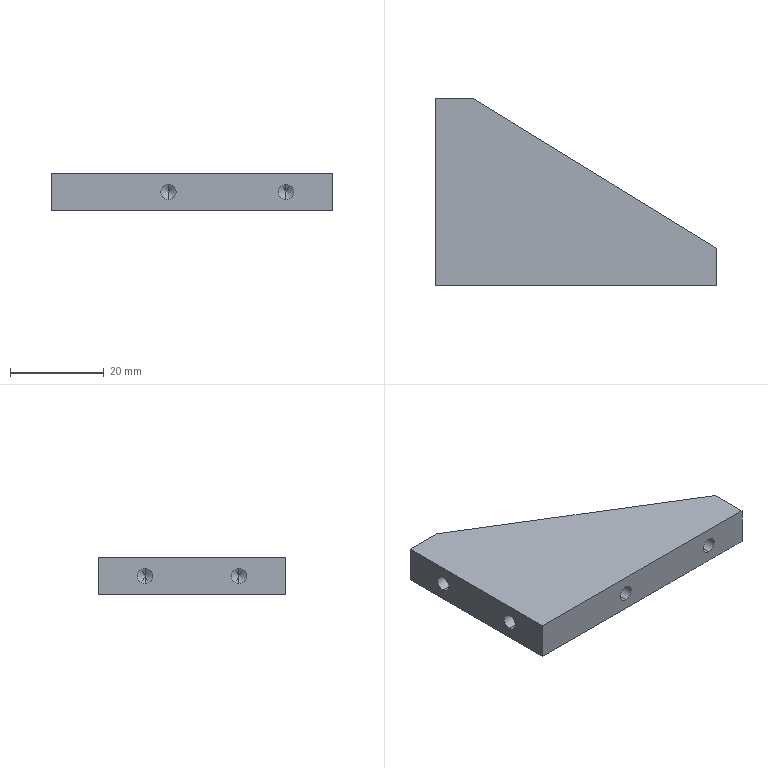Part | STEP file | 2072 Cylinder reinforcing rib plate | 1 solid | 23 faces | box 60 x 40 x 8 mm | volume 12139 mm3 | cylinder 8 | cone 8 | plane 7 | commonest cylinder face diameters 3.3 x8
STEP:
#1=CARTESIAN_POINT('',(0.,0.,0.));
#2=DIRECTION('',(0.,0.,1.));
#3=DIRECTION('',(1.,0.,0.));
#4=AXIS2_PLACEMENT_3D('',#1,#2,#3);
#5=CARTESIAN_POINT('',(25.,11.5,2.35));
#6=VERTEX_POINT('',#5);
#7=CARTESIAN_POINT('',(25.,0.,2.35));
#8=VERTEX_POINT('',#7);
#9=CARTESIAN_POINT('',(25.,0.,2.35));
#10=DIRECTION('',(0.,-1.,0.));
#11=VECTOR('',#10,1.);
#12=LINE('',#9,#11);
#13=CARTESIAN_POINT('',(25.,0.,4.));
#14=DIRECTION('',(0.,-1.,0.));
#15=DIRECTION('',(0.,0.,-1.));
#16=AXIS2_PLACEMENT_3D('',#13,#14,#15);
#17=CYLINDRICAL_SURFACE('',#16,1.65);
#18=CARTESIAN_POINT('',(6.283,0.));
#19=DIRECTION('',(0.,1.));
#20=VECTOR('',#19,1.);
#21=LINE('',#18,#20);
#22=(GEOMETRIC_REPRESENTATION_CONTEXT(2)PARAMETRIC_REPRESENTATION_CONTEXT()REPRESENTATION_CONTEXT('',''));
#23=DEFINITIONAL_REPRESENTATION('',(#21),#22);
#24=PCURVE('',#17,#23);
#25=CARTESIAN_POINT('',(25.,0.,4.));
#26=DIRECTION('',(0.,-1.,0.));
#27=DIRECTION('',(0.,0.,-1.));
#28=AXIS2_PLACEMENT_3D('',#25,#26,#27);
#29=CYLINDRICAL_SURFACE('',#28,1.65);
#30=CARTESIAN_POINT('',(0.,0.));
#31=DIRECTION('',(0.,1.));
#32=VECTOR('',#31,1.);
#33=LINE('',#30,#32);
#34=(GEOMETRIC_REPRESENTATION_CONTEXT(2)PARAMETRIC_REPRESENTATION_CONTEXT()REPRESENTATION_CONTEXT('',''));
#35=DEFINITIONAL_REPRESENTATION('',(#33),#34);
#36=PCURVE('',#29,#35);
#37=SURFACE_CURVE('',#12,(#24,#36),.PCURVE_S1.);
#38=EDGE_CURVE('',#6,#8,#37,.T.);
#39=ORIENTED_EDGE('',*,*,#38,.T.);
#40=CARTESIAN_POINT('',(25.,0.,5.65));
#41=VERTEX_POINT('',#40);
#42=CARTESIAN_POINT('',(25.,0.,4.));
#43=DIRECTION('',(0.,-1.,0.));
#44=DIRECTION('',(0.,0.,-1.));
#45=AXIS2_PLACEMENT_3D('',#42,#43,#44);
#46=CIRCLE('',#45,1.65);
#47=CARTESIAN_POINT('',(0.,0.));
#48=DIRECTION('',(1.,0.));
#49=VECTOR('',#48,1.);
#50=LINE('',#47,#49);
#51=(GEOMETRIC_REPRESENTATION_CONTEXT(2)PARAMETRIC_REPRESENTATION_CONTEXT()REPRESENTATION_CONTEXT('',''));
#52=DEFINITIONAL_REPRESENTATION('',(#50),#51);
#53=PCURVE('',#17,#52);
#54=CARTESIAN_POINT('',(0.,0.,8.));
#55=DIRECTION('',(0.,1.,0.));
#56=DIRECTION('',(0.,0.,1.));
#57=AXIS2_PLACEMENT_3D('',#54,#55,#56);
#58=PLANE('',#57);
#59=CARTESIAN_POINT('',(-5.65,25.));
#60=CARTESIAN_POINT('',(-5.65,27.858));
#61=CARTESIAN_POINT('',(-3.175,26.429));
#62=CARTESIAN_POINT('',(-0.7,25.));
#63=CARTESIAN_POINT('',(-3.175,23.571));
#64=CARTESIAN_POINT('',(-5.65,22.142));
#65=CARTESIAN_POINT('',(-5.65,25.));
#66=(BOUNDED_CURVE()B_SPLINE_CURVE(2,(#59,#60,#61,#62,#63,#64,#65),.UNSPECIFIED.,.T.,.F.)B_SPLINE_CURVE_WITH_KNOTS((1,2,2,2,2,1),(-2.094,0.,2.094,4.189,6.283,8.378),.UNSPECIFIED.)CURVE()GEOMETRIC_REPRESENTATION_ITEM()RATIONAL_B_SPLINE_CURVE((1.,0.5,1.,0.5,1.,0.5,1.))REPRESENTATION_ITEM(''));
#67=(GEOMETRIC_REPRESENTATION_CONTEXT(2)PARAMETRIC_REPRESENTATION_CONTEXT()REPRESENTATION_CONTEXT('',''));
#68=DEFINITIONAL_REPRESENTATION('',(#66),#67);
#69=PCURVE('',#58,#68);
#70=SURFACE_CURVE('',#46,(#53,#69),.PCURVE_S1.);
#71=EDGE_CURVE('',#41,#8,#70,.T.);
#72=ORIENTED_EDGE('',*,*,#71,.F.);
#73=CARTESIAN_POINT('',(25.,11.5,5.65));
#74=VERTEX_POINT('',#73);
#75=CARTESIAN_POINT('',(25.,0.,5.65));
#76=DIRECTION('',(0.,-1.,0.));
#77=VECTOR('',#76,1.);
#78=LINE('',#75,#77);
#79=CARTESIAN_POINT('',(3.142,0.));
#80=DIRECTION('',(0.,1.));
#81=VECTOR('',#80,1.);
#82=LINE('',#79,#81);
#83=(GEOMETRIC_REPRESENTATION_CONTEXT(2)PARAMETRIC_REPRESENTATION_CONTEXT()REPRESENTATION_CONTEXT('',''));
#84=DEFINITIONAL_REPRESENTATION('',(#82),#83);
#85=PCURVE('',#17,#84);
#86=CARTESIAN_POINT('',(3.142,0.));
#87=DIRECTION('',(0.,1.));
#88=VECTOR('',#87,1.);
#89=LINE('',#86,#88);
#90=(GEOMETRIC_REPRESENTATION_CONTEXT(2)PARAMETRIC_REPRESENTATION_CONTEXT()REPRESENTATION_CONTEXT('',''));
#91=DEFINITIONAL_REPRESENTATION('',(#89),#90);
#92=PCURVE('',#29,#91);
#93=SURFACE_CURVE('',#78,(#85,#92),.PCURVE_S1.);
#94=EDGE_CURVE('',#74,#41,#93,.T.);
#95=ORIENTED_EDGE('',*,*,#94,.F.);
#96=CARTESIAN_POINT('',(25.,11.5,4.));
#97=DIRECTION('',(0.,-1.,0.));
#98=DIRECTION('',(0.,0.,-1.));
#99=AXIS2_PLACEMENT_3D('',#96,#97,#98);
#100=CIRCLE('',#99,1.65);
#101=CARTESIAN_POINT('',(0.,-11.5));
#102=DIRECTION('',(1.,0.));
#103=VECTOR('',#102,1.);
#104=LINE('',#101,#103);
#105=(GEOMETRIC_REPRESENTATION_CONTEXT(2)PARAMETRIC_REPRESENTATION_CONTEXT()REPRESENTATION_CONTEXT('',''));
#106=DEFINITIONAL_REPRESENTATION('',(#104),#105);
#107=PCURVE('',#17,#106);
#108=CARTESIAN_POINT('',(25.,11.5,4.));
#109=DIRECTION('',(0.,-1.,0.));
#110=DIRECTION('',(0.,0.,-1.));
#111=AXIS2_PLACEMENT_3D('',#108,#109,#110);
#112=CONICAL_SURFACE('',#111,1.65,1.03);
#113=CARTESIAN_POINT('',(0.,0.));
#114=DIRECTION('',(1.,0.));
#115=VECTOR('',#114,1.);
#116=LINE('',#113,#115);
#117=(GEOMETRIC_REPRESENTATION_CONTEXT(2)PARAMETRIC_REPRESENTATION_CONTEXT()REPRESENTATION_CONTEXT('',''));
#118=DEFINITIONAL_REPRESENTATION('',(#116),#117);
#119=PCURVE('',#112,#118);
#120=SURFACE_CURVE('',#100,(#107,#119),.PCURVE_S1.);
#121=EDGE_CURVE('',#74,#6,#120,.T.);
#122=ORIENTED_EDGE('',*,*,#121,.T.);
#123=EDGE_LOOP('',(#39,#72,#95,#122));
#124=FACE_BOUND('',#123,.F.);
#125=ADVANCED_FACE('',(#124),#17,.F.);
#126=ORIENTED_EDGE('',*,*,#121,.F.);
#127=CARTESIAN_POINT('',(25.,12.491,4.));
#128=VERTEX_POINT('',#127);
#129=CARTESIAN_POINT('',(25.,11.5,5.65));
#130=DIRECTION('',(0.,-0.515,0.8572));
#131=VECTOR('',#130,1.);
#132=LINE('',#129,#131);
#133=CARTESIAN_POINT('',(3.142,0.));
#134=DIRECTION('',(0.,1.));
#135=VECTOR('',#134,1.);
#136=LINE('',#133,#135);
#137=(GEOMETRIC_REPRESENTATION_CONTEXT(2)PARAMETRIC_REPRESENTATION_CONTEXT()REPRESENTATION_CONTEXT('',''));
#138=DEFINITIONAL_REPRESENTATION('',(#136),#137);
#139=PCURVE('',#112,#138);
#140=CARTESIAN_POINT('',(25.,11.5,4.));
#141=DIRECTION('',(0.,-1.,0.));
#142=DIRECTION('',(0.,0.,-1.));
#143=AXIS2_PLACEMENT_3D('',#140,#141,#142);
#144=CONICAL_SURFACE('',#143,1.65,1.03);
#145=CARTESIAN_POINT('',(3.142,0.));
#146=DIRECTION('',(0.,1.));
#147=VECTOR('',#146,1.);
#148=LINE('',#145,#147);
#149=(GEOMETRIC_REPRESENTATION_CONTEXT(2)PARAMETRIC_REPRESENTATION_CONTEXT()REPRESENTATION_CONTEXT('',''));
#150=DEFINITIONAL_REPRESENTATION('',(#148),#149);
#151=PCURVE('',#144,#150);
#152=SURFACE_CURVE('',#132,(#139,#151),.PCURVE_S1.);
#153=EDGE_CURVE('',#128,#74,#152,.T.);
#154=ORIENTED_EDGE('',*,*,#153,.F.);
#155=CARTESIAN_POINT('',(25.,11.5,2.35));
#156=DIRECTION('',(0.,-0.515,-0.8572));
#157=VECTOR('',#156,1.);
#158=LINE('',#155,#157);
#159=CARTESIAN_POINT('',(6.283,0.));
#160=DIRECTION('',(0.,1.));
#161=VECTOR('',#160,1.);
#162=LINE('',#159,#161);
#163=(GEOMETRIC_REPRESENTATION_CONTEXT(2)PARAMETRIC_REPRESENTATION_CONTEXT()REPRESENTATION_CONTEXT('',''));
#164=DEFINITIONAL_REPRESENTATION('',(#162),#163);
#165=PCURVE('',#112,#164);
#166=CARTESIAN_POINT('',(0.,0.));
#167=DIRECTION('',(0.,1.));
#168=VECTOR('',#167,1.);
#169=LINE('',#166,#168);
#170=(GEOMETRIC_REPRESENTATION_CONTEXT(2)PARAMETRIC_REPRESENTATION_CONTEXT()REPRESENTATION_CONTEXT('',''));
#171=DEFINITIONAL_REPRESENTATION('',(#169),#170);
#172=PCURVE('',#144,#171);
#173=SURFACE_CURVE('',#158,(#165,#172),.PCURVE_S1.);
#174=EDGE_CURVE('',#128,#6,#173,.T.);
#175=ORIENTED_EDGE('',*,*,#174,.T.);
#176=EDGE_LOOP('',(#126,#154,#175));
#177=FACE_BOUND('',#176,.F.);
#178=ADVANCED_FACE('',(#177),#112,.F.);
#179=CARTESIAN_POINT('',(50.,11.5,2.35));
#180=VERTEX_POINT('',#179);
#181=CARTESIAN_POINT('',(50.,0.,2.35));
#182=VERTEX_POINT('',#181);
#183=CARTESIAN_POINT('',(50.,0.,2.35));
#184=DIRECTION('',(0.,-1.,0.));
#185=VECTOR('',#184,1.);
#186=LINE('',#183,#185);
#187=CARTESIAN_POINT('',(50.,0.,4.));
#188=DIRECTION('',(0.,-1.,0.));
#189=DIRECTION('',(0.,0.,-1.));
#190=AXIS2_PLACEMENT_3D('',#187,#188,#189);
#191=CYLINDRICAL_SURFACE('',#190,1.65);
#192=CARTESIAN_POINT('',(6.283,0.));
#193=DIRECTION('',(0.,1.));
#194=VECTOR('',#193,1.);
#195=LINE('',#192,#194);
#196=(GEOMETRIC_REPRESENTATION_CONTEXT(2)PARAMETRIC_REPRESENTATION_CONTEXT()REPRESENTATION_CONTEXT('',''));
#197=DEFINITIONAL_REPRESENTATION('',(#195),#196);
#198=PCURVE('',#191,#197);
#199=CARTESIAN_POINT('',(50.,0.,4.));
#200=DIRECTION('',(0.,-1.,0.));
#201=DIRECTION('',(0.,0.,-1.));
#202=AXIS2_PLACEMENT_3D('',#199,#200,#201);
#203=CYLINDRICAL_SURFACE('',#202,1.65);
#204=CARTESIAN_POINT('',(0.,0.));
#205=DIRECTION('',(0.,1.));
#206=VECTOR('',#205,1.);
#207=LINE('',#204,#206);
#208=(GEOMETRIC_REPRESENTATION_CONTEXT(2)PARAMETRIC_REPRESENTATION_CONTEXT()REPRESENTATION_CONTEXT('',''));
#209=DEFINITIONAL_REPRESENTATION('',(#207),#208);
#210=PCURVE('',#203,#209);
#211=SURFACE_CURVE('',#186,(#198,#210),.PCURVE_S1.);
#212=EDGE_CURVE('',#180,#182,#211,.T.);
#213=ORIENTED_EDGE('',*,*,#212,.T.);
#214=CARTESIAN_POINT('',(50.,0.,5.65));
#215=VERTEX_POINT('',#214);
#216=CARTESIAN_POINT('',(50.,0.,4.));
#217=DIRECTION('',(0.,-1.,0.));
#218=DIRECTION('',(0.,0.,-1.));
#219=AXIS2_PLACEMENT_3D('',#216,#217,#218);
#220=CIRCLE('',#219,1.65);
#221=CARTESIAN_POINT('',(0.,0.));
#222=DIRECTION('',(1.,0.));
#223=VECTOR('',#222,1.);
#224=LINE('',#221,#223);
#225=(GEOMETRIC_REPRESENTATION_CONTEXT(2)PARAMETRIC_REPRESENTATION_CONTEXT()REPRESENTATION_CONTEXT('',''));
#226=DEFINITIONAL_REPRESENTATION('',(#224),#225);
#227=PCURVE('',#191,#226);
#228=CARTESIAN_POINT('',(-5.65,50.));
#229=CARTESIAN_POINT('',(-5.65,52.858));
#230=CARTESIAN_POINT('',(-3.175,51.429));
#231=CARTESIAN_POINT('',(-0.7,50.));
#232=CARTESIAN_POINT('',(-3.175,48.571));
#233=CARTESIAN_POINT('',(-5.65,47.142));
#234=CARTESIAN_POINT('',(-5.65,50.));
#235=(BOUNDED_CURVE()B_SPLINE_CURVE(2,(#228,#229,#230,#231,#232,#233,#234),.UNSPECIFIED.,.T.,.F.)B_SPLINE_CURVE_WITH_KNOTS((1,2,2,2,2,1),(-2.094,0.,2.094,4.189,6.283,8.378),.UNSPECIFIED.)CURVE()GEOMETRIC_REPRESENTATION_ITEM()RATIONAL_B_SPLINE_CURVE((1.,0.5,1.,0.5,1.,0.5,1.))REPRESENTATION_ITEM(''));
#236=(GEOMETRIC_REPRESENTATION_CONTEXT(2)PARAMETRIC_REPRESENTATION_CONTEXT()REPRESENTATION_CONTEXT('',''));
#237=DEFINITIONAL_REPRESENTATION('',(#235),#236);
#238=PCURVE('',#58,#237);
#239=SURFACE_CURVE('',#220,(#227,#238),.PCURVE_S1.);
#240=EDGE_CURVE('',#215,#182,#239,.T.);
#241=ORIENTED_EDGE('',*,*,#240,.F.);
#242=CARTESIAN_POINT('',(50.,11.5,5.65));
#243=VERTEX_POINT('',#242);
#244=CARTESIAN_POINT('',(50.,0.,5.65));
#245=DIRECTION('',(0.,-1.,0.));
#246=VECTOR('',#245,1.);
#247=LINE('',#244,#246);
#248=CARTESIAN_POINT('',(3.142,0.));
#249=DIRECTION('',(0.,1.));
#250=VECTOR('',#249,1.);
#251=LINE('',#248,#250);
#252=(GEOMETRIC_REPRESENTATION_CONTEXT(2)PARAMETRIC_REPRESENTATION_CONTEXT()REPRESENTATION_CONTEXT('',''));
#253=DEFINITIONAL_REPRESENTATION('',(#251),#252);
#254=PCURVE('',#191,#253);
#255=CARTESIAN_POINT('',(3.142,0.));
#256=DIRECTION('',(0.,1.));
#257=VECTOR('',#256,1.);
#258=LINE('',#255,#257);
#259=(GEOMETRIC_REPRESENTATION_CONTEXT(2)PARAMETRIC_REPRESENTATION_CONTEXT()REPRESENTATION_CONTEXT('',''));
#260=DEFINITIONAL_REPRESENTATION('',(#258),#259);
#261=PCURVE('',#203,#260);
#262=SURFACE_CURVE('',#247,(#254,#261),.PCURVE_S1.);
#263=EDGE_CURVE('',#243,#215,#262,.T.);
#264=ORIENTED_EDGE('',*,*,#263,.F.);
#265=CARTESIAN_POINT('',(50.,11.5,4.));
#266=DIRECTION('',(0.,-1.,0.));
#267=DIRECTION('',(0.,0.,-1.));
#268=AXIS2_PLACEMENT_3D('',#265,#266,#267);
#269=CIRCLE('',#268,1.65);
#270=CARTESIAN_POINT('',(0.,-11.5));
#271=DIRECTION('',(1.,0.));
#272=VECTOR('',#271,1.);
#273=LINE('',#270,#272);
#274=(GEOMETRIC_REPRESENTATION_CONTEXT(2)PARAMETRIC_REPRESENTATION_CONTEXT()REPRESENTATION_CONTEXT('',''));
#275=DEFINITIONAL_REPRESENTATION('',(#273),#274);
#276=PCURVE('',#191,#275);
#277=CARTESIAN_POINT('',(50.,11.5,4.));
#278=DIRECTION('',(0.,-1.,0.));
#279=DIRECTION('',(0.,0.,-1.));
#280=AXIS2_PLACEMENT_3D('',#277,#278,#279);
#281=CONICAL_SURFACE('',#280,1.65,1.03);
#282=CARTESIAN_POINT('',(0.,0.));
#283=DIRECTION('',(1.,0.));
#284=VECTOR('',#283,1.);
#285=LINE('',#282,#284);
#286=(GEOMETRIC_REPRESENTATION_CONTEXT(2)PARAMETRIC_REPRESENTATION_CONTEXT()REPRESENTATION_CONTEXT('',''));
#287=DEFINITIONAL_REPRESENTATION('',(#285),#286);
#288=PCURVE('',#281,#287);
#289=SURFACE_CURVE('',#269,(#276,#288),.PCURVE_S1.);
#290=EDGE_CURVE('',#243,#180,#289,.T.);
#291=ORIENTED_EDGE('',*,*,#290,.T.);
#292=EDGE_LOOP('',(#213,#241,#264,#291));
#293=FACE_BOUND('',#292,.F.);
#294=ADVANCED_FACE('',(#293),#191,.F.);
#295=ORIENTED_EDGE('',*,*,#290,.F.);
#296=CARTESIAN_POINT('',(50.,12.491,4.));
#297=VERTEX_POINT('',#296);
#298=CARTESIAN_POINT('',(50.,11.5,5.65));
#299=DIRECTION('',(0.,-0.515,0.8572));
#300=VECTOR('',#299,1.);
#301=LINE('',#298,#300);
#302=CARTESIAN_POINT('',(3.142,-0.9914));
#303=CARTESIAN_POINT('',(3.142,-0.9764));
#304=CARTESIAN_POINT('',(3.142,-0.9464));
#305=CARTESIAN_POINT('',(3.142,-0.9013));
#306=CARTESIAN_POINT('',(3.142,-0.8562));
#307=CARTESIAN_POINT('',(3.142,-0.8112));
#308=CARTESIAN_POINT('',(3.142,-0.7661));
#309=CARTESIAN_POINT('',(3.142,-0.721));
#310=CARTESIAN_POINT('',(3.142,-0.676));
#311=CARTESIAN_POINT('',(3.142,-0.6309));
#312=CARTESIAN_POINT('',(3.142,-0.5858));
#313=CARTESIAN_POINT('',(3.142,-0.5408));
#314=CARTESIAN_POINT('',(3.142,-0.4957));
#315=CARTESIAN_POINT('',(3.142,-0.4506));
#316=CARTESIAN_POINT('',(3.142,-0.4056));
#317=CARTESIAN_POINT('',(3.142,-0.3605));
#318=CARTESIAN_POINT('',(3.142,-0.3155));
#319=CARTESIAN_POINT('',(3.142,-0.2704));
#320=CARTESIAN_POINT('',(3.142,-0.2253));
#321=CARTESIAN_POINT('',(3.142,-0.1803));
#322=CARTESIAN_POINT('',(3.142,-0.1352));
#323=CARTESIAN_POINT('',(3.142,-0.09013));
#324=CARTESIAN_POINT('',(3.142,-0.04506));
#325=CARTESIAN_POINT('',(3.142,-0.01502));
#326=CARTESIAN_POINT('',(3.142,0.));
#327=B_SPLINE_CURVE_WITH_KNOTS('',3,(#302,#303,#304,#305,#306,#307,#308,#309,#310,#311,#312,#313,#314,#315,#316,#317,#318,#319,#320,#321,#322,#323,#324,#325,#326),.UNSPECIFIED.,.F.,.F.,(4,1,1,1,1,1,1,1,1,1,1,1,1,1,1,1,1,1,1,1,1,1,4),(-1.925,-1.837,-1.75,-1.662,-1.575,-1.487,-1.4,-1.312,-1.225,-1.137,-1.05,-0.9625,-0.875,-0.7875,-0.7,-0.6125,-0.525,-0.4375,-0.35,-0.2625,-0.175,-0.0875,0.),.UNSPECIFIED.);
#328=(GEOMETRIC_REPRESENTATION_CONTEXT(2)PARAMETRIC_REPRESENTATION_CONTEXT()REPRESENTATION_CONTEXT('',''));
#329=DEFINITIONAL_REPRESENTATION('',(#327),#328);
#330=PCURVE('',#281,#329);
#331=CARTESIAN_POINT('',(50.,11.5,4.));
#332=DIRECTION('',(0.,-1.,0.));
#333=DIRECTION('',(0.,0.,-1.));
#334=AXIS2_PLACEMENT_3D('',#331,#332,#333);
#335=CONICAL_SURFACE('',#334,1.65,1.03);
#336=CARTESIAN_POINT('',(3.142,-0.9914));
#337=CARTESIAN_POINT('',(3.142,-0.9764));
#338=CARTESIAN_POINT('',(3.142,-0.9464));
#339=CARTESIAN_POINT('',(3.142,-0.9013));
#340=CARTESIAN_POINT('',(3.142,-0.8562));
#341=CARTESIAN_POINT('',(3.142,-0.8112));
#342=CARTESIAN_POINT('',(3.142,-0.7661));
#343=CARTESIAN_POINT('',(3.142,-0.721));
#344=CARTESIAN_POINT('',(3.142,-0.676));
#345=CARTESIAN_POINT('',(3.142,-0.6309));
#346=CARTESIAN_POINT('',(3.142,-0.5858));
#347=CARTESIAN_POINT('',(3.142,-0.5408));
#348=CARTESIAN_POINT('',(3.142,-0.4957));
#349=CARTESIAN_POINT('',(3.142,-0.4506));
#350=CARTESIAN_POINT('',(3.142,-0.4056));
#351=CARTESIAN_POINT('',(3.142,-0.3605));
#352=CARTESIAN_POINT('',(3.142,-0.3155));
#353=CARTESIAN_POINT('',(3.142,-0.2704));
#354=CARTESIAN_POINT('',(3.142,-0.2253));
#355=CARTESIAN_POINT('',(3.142,-0.1803));
#356=CARTESIAN_POINT('',(3.142,-0.1352));
#357=CARTESIAN_POINT('',(3.142,-0.09013));
#358=CARTESIAN_POINT('',(3.142,-0.04506));
#359=CARTESIAN_POINT('',(3.142,-0.01502));
#360=CARTESIAN_POINT('',(3.142,0.));
#361=B_SPLINE_CURVE_WITH_KNOTS('',3,(#336,#337,#338,#339,#340,#341,#342,#343,#344,#345,#346,#347,#348,#349,#350,#351,#352,#353,#354,#355,#356,#357,#358,#359,#360),.UNSPECIFIED.,.F.,.F.,(4,1,1,1,1,1,1,1,1,1,1,1,1,1,1,1,1,1,1,1,1,1,4),(-1.925,-1.837,-1.75,-1.662,-1.575,-1.487,-1.4,-1.312,-1.225,-1.137,-1.05,-0.9625,-0.875,-0.7875,-0.7,-0.6125,-0.525,-0.4375,-0.35,-0.2625,-0.175,-0.0875,0.),.UNSPECIFIED.);
#362=(GEOMETRIC_REPRESENTATION_CONTEXT(2)PARAMETRIC_REPRESENTATION_CONTEXT()REPRESENTATION_CONTEXT('',''));
#363=DEFINITIONAL_REPRESENTATION('',(#361),#362);
#364=PCURVE('',#335,#363);
#365=SURFACE_CURVE('',#301,(#330,#364),.PCURVE_S1.);
#366=EDGE_CURVE('',#297,#243,#365,.T.);
#367=ORIENTED_EDGE('',*,*,#366,.F.);
#368=CARTESIAN_POINT('',(50.,11.5,2.35));
#369=DIRECTION('',(0.,-0.515,-0.8572));
#370=VECTOR('',#369,1.);
#371=LINE('',#368,#370);
#372=CARTESIAN_POINT('',(6.283,0.));
#373=DIRECTION('',(0.,1.));
#374=VECTOR('',#373,1.);
#375=LINE('',#372,#374);
#376=(GEOMETRIC_REPRESENTATION_CONTEXT(2)PARAMETRIC_REPRESENTATION_CONTEXT()REPRESENTATION_CONTEXT('',''));
#377=DEFINITIONAL_REPRESENTATION('',(#375),#376);
#378=PCURVE('',#281,#377);
#379=CARTESIAN_POINT('',(0.,0.));
#380=DIRECTION('',(0.,1.));
#381=VECTOR('',#380,1.);
#382=LINE('',#379,#381);
#383=(GEOMETRIC_REPRESENTATION_CONTEXT(2)PARAMETRIC_REPRESENTATION_CONTEXT()REPRESENTATION_CONTEXT('',''));
#384=DEFINITIONAL_REPRESENTATION('',(#382),#383);
#385=PCURVE('',#335,#384);
#386=SURFACE_CURVE('',#371,(#378,#385),.PCURVE_S1.);
#387=EDGE_CURVE('',#297,#180,#386,.T.);
#388=ORIENTED_EDGE('',*,*,#387,.T.);
#389=EDGE_LOOP('',(#295,#367,#388));
#390=FACE_BOUND('',#389,.F.);
#391=ADVANCED_FACE('',(#390),#281,.F.);
#392=CARTESIAN_POINT('',(11.5,10.,5.65));
#393=VERTEX_POINT('',#392);
#394=CARTESIAN_POINT('',(0.,10.,5.65));
#395=VERTEX_POINT('',#394);
#396=CARTESIAN_POINT('',(0.,10.,5.65));
#397=DIRECTION('',(-1.,0.,0.));
#398=VECTOR('',#397,1.);
#399=LINE('',#396,#398);
#400=CARTESIAN_POINT('',(0.,10.,4.));
#401=DIRECTION('',(-1.,0.,0.));
#402=DIRECTION('',(0.,0.,1.));
#403=AXIS2_PLACEMENT_3D('',#400,#401,#402);
#404=CYLINDRICAL_SURFACE('',#403,1.65);
#405=CARTESIAN_POINT('',(6.283,0.));
#406=DIRECTION('',(0.,1.));
#407=VECTOR('',#406,1.);
#408=LINE('',#405,#407);
#409=(GEOMETRIC_REPRESENTATION_CONTEXT(2)PARAMETRIC_REPRESENTATION_CONTEXT()REPRESENTATION_CONTEXT('',''));
#410=DEFINITIONAL_REPRESENTATION('',(#408),#409);
#411=PCURVE('',#404,#410);
#412=CARTESIAN_POINT('',(0.,10.,4.));
#413=DIRECTION('',(-1.,0.,0.));
#414=DIRECTION('',(0.,0.,1.));
#415=AXIS2_PLACEMENT_3D('',#412,#413,#414);
#416=CYLINDRICAL_SURFACE('',#415,1.65);
#417=CARTESIAN_POINT('',(0.,0.));
#418=DIRECTION('',(0.,1.));
#419=VECTOR('',#418,1.);
#420=LINE('',#417,#419);
#421=(GEOMETRIC_REPRESENTATION_CONTEXT(2)PARAMETRIC_REPRESENTATION_CONTEXT()REPRESENTATION_CONTEXT('',''));
#422=DEFINITIONAL_REPRESENTATION('',(#420),#421);
#423=PCURVE('',#416,#422);
#424=SURFACE_CURVE('',#399,(#411,#423),.PCURVE_S1.);
#425=EDGE_CURVE('',#393,#395,#424,.T.);
#426=ORIENTED_EDGE('',*,*,#425,.T.);
#427=CARTESIAN_POINT('',(0.,10.,2.35));
#428=VERTEX_POINT('',#427);
#429=CARTESIAN_POINT('',(0.,10.,4.));
#430=DIRECTION('',(-1.,0.,0.));
#431=DIRECTION('',(0.,0.,1.));
#432=AXIS2_PLACEMENT_3D('',#429,#430,#431);
#433=CIRCLE('',#432,1.65);
#434=CARTESIAN_POINT('',(0.,0.));
#435=DIRECTION('',(1.,0.));
#436=VECTOR('',#435,1.);
#437=LINE('',#434,#436);
#438=(GEOMETRIC_REPRESENTATION_CONTEXT(2)PARAMETRIC_REPRESENTATION_CONTEXT()REPRESENTATION_CONTEXT('',''));
#439=DEFINITIONAL_REPRESENTATION('',(#437),#438);
#440=PCURVE('',#404,#439);
#441=CARTESIAN_POINT('',(0.,40.,8.));
#442=DIRECTION('',(1.,0.,0.));
#443=DIRECTION('',(0.,0.,-1.));
#444=AXIS2_PLACEMENT_3D('',#441,#442,#443);
#445=PLANE('',#444);
#446=CARTESIAN_POINT('',(2.35,-30.));
#447=CARTESIAN_POINT('',(2.35,-27.142));
#448=CARTESIAN_POINT('',(4.825,-28.571));
#449=CARTESIAN_POINT('',(7.3,-30.));
#450=CARTESIAN_POINT('',(4.825,-31.429));
#451=CARTESIAN_POINT('',(2.35,-32.858));
#452=CARTESIAN_POINT('',(2.35,-30.));
#453=(BOUNDED_CURVE()B_SPLINE_CURVE(2,(#446,#447,#448,#449,#450,#451,#452),.UNSPECIFIED.,.T.,.F.)B_SPLINE_CURVE_WITH_KNOTS((1,2,2,2,2,1),(-2.094,0.,2.094,4.189,6.283,8.378),.UNSPECIFIED.)CURVE()GEOMETRIC_REPRESENTATION_ITEM()RATIONAL_B_SPLINE_CURVE((1.,0.5,1.,0.5,1.,0.5,1.))REPRESENTATION_ITEM(''));
#454=(GEOMETRIC_REPRESENTATION_CONTEXT(2)PARAMETRIC_REPRESENTATION_CONTEXT()REPRESENTATION_CONTEXT('',''));
#455=DEFINITIONAL_REPRESENTATION('',(#453),#454);
#456=PCURVE('',#445,#455);
#457=SURFACE_CURVE('',#433,(#440,#456),.PCURVE_S1.);
#458=EDGE_CURVE('',#428,#395,#457,.T.);
#459=ORIENTED_EDGE('',*,*,#458,.F.);
#460=CARTESIAN_POINT('',(11.5,10.,2.35));
#461=VERTEX_POINT('',#460);
#462=CARTESIAN_POINT('',(0.,10.,2.35));
#463=DIRECTION('',(-1.,0.,0.));
#464=VECTOR('',#463,1.);
#465=LINE('',#462,#464);
#466=CARTESIAN_POINT('',(3.142,0.));
#467=DIRECTION('',(0.,1.));
#468=VECTOR('',#467,1.);
#469=LINE('',#466,#468);
#470=(GEOMETRIC_REPRESENTATION_CONTEXT(2)PARAMETRIC_REPRESENTATION_CONTEXT()REPRESENTATION_CONTEXT('',''));
#471=DEFINITIONAL_REPRESENTATION('',(#469),#470);
#472=PCURVE('',#404,#471);
#473=CARTESIAN_POINT('',(3.142,0.));
#474=DIRECTION('',(0.,1.));
#475=VECTOR('',#474,1.);
#476=LINE('',#473,#475);
#477=(GEOMETRIC_REPRESENTATION_CONTEXT(2)PARAMETRIC_REPRESENTATION_CONTEXT()REPRESENTATION_CONTEXT('',''));
#478=DEFINITIONAL_REPRESENTATION('',(#476),#477);
#479=PCURVE('',#416,#478);
#480=SURFACE_CURVE('',#465,(#472,#479),.PCURVE_S1.);
#481=EDGE_CURVE('',#461,#428,#480,.T.);
#482=ORIENTED_EDGE('',*,*,#481,.F.);
#483=CARTESIAN_POINT('',(11.5,10.,4.));
#484=DIRECTION('',(-1.,0.,0.));
#485=DIRECTION('',(0.,0.,1.));
#486=AXIS2_PLACEMENT_3D('',#483,#484,#485);
#487=CIRCLE('',#486,1.65);
#488=CARTESIAN_POINT('',(0.,-11.5));
#489=DIRECTION('',(1.,0.));
#490=VECTOR('',#489,1.);
#491=LINE('',#488,#490);
#492=(GEOMETRIC_REPRESENTATION_CONTEXT(2)PARAMETRIC_REPRESENTATION_CONTEXT()REPRESENTATION_CONTEXT('',''));
#493=DEFINITIONAL_REPRESENTATION('',(#491),#492);
#494=PCURVE('',#404,#493);
#495=CARTESIAN_POINT('',(11.5,10.,4.));
#496=DIRECTION('',(-1.,0.,0.));
#497=DIRECTION('',(0.,0.,1.));
#498=AXIS2_PLACEMENT_3D('',#495,#496,#497);
#499=CONICAL_SURFACE('',#498,1.65,1.03);
#500=CARTESIAN_POINT('',(0.,0.));
#501=DIRECTION('',(1.,0.));
#502=VECTOR('',#501,1.);
#503=LINE('',#500,#502);
#504=(GEOMETRIC_REPRESENTATION_CONTEXT(2)PARAMETRIC_REPRESENTATION_CONTEXT()REPRESENTATION_CONTEXT('',''));
#505=DEFINITIONAL_REPRESENTATION('',(#503),#504);
#506=PCURVE('',#499,#505);
#507=SURFACE_CURVE('',#487,(#494,#506),.PCURVE_S1.);
#508=EDGE_CURVE('',#461,#393,#507,.T.);
#509=ORIENTED_EDGE('',*,*,#508,.T.);
#510=EDGE_LOOP('',(#426,#459,#482,#509));
#511=FACE_BOUND('',#510,.F.);
#512=ADVANCED_FACE('',(#511),#404,.F.);
#513=ORIENTED_EDGE('',*,*,#508,.F.);
#514=CARTESIAN_POINT('',(12.491,10.,4.));
#515=VERTEX_POINT('',#514);
#516=CARTESIAN_POINT('',(11.5,10.,2.35));
#517=DIRECTION('',(-0.515,0.,-0.8572));
#518=VECTOR('',#517,1.);
#519=LINE('',#516,#518);
#520=CARTESIAN_POINT('',(3.142,0.));
#521=DIRECTION('',(0.,1.));
#522=VECTOR('',#521,1.);
#523=LINE('',#520,#522);
#524=(GEOMETRIC_REPRESENTATION_CONTEXT(2)PARAMETRIC_REPRESENTATION_CONTEXT()REPRESENTATION_CONTEXT('',''));
#525=DEFINITIONAL_REPRESENTATION('',(#523),#524);
#526=PCURVE('',#499,#525);
#527=CARTESIAN_POINT('',(11.5,10.,4.));
#528=DIRECTION('',(-1.,0.,0.));
#529=DIRECTION('',(0.,0.,1.));
#530=AXIS2_PLACEMENT_3D('',#527,#528,#529);
#531=CONICAL_SURFACE('',#530,1.65,1.03);
#532=CARTESIAN_POINT('',(3.142,0.));
#533=DIRECTION('',(0.,1.));
#534=VECTOR('',#533,1.);
#535=LINE('',#532,#534);
#536=(GEOMETRIC_REPRESENTATION_CONTEXT(2)PARAMETRIC_REPRESENTATION_CONTEXT()REPRESENTATION_CONTEXT('',''));
#537=DEFINITIONAL_REPRESENTATION('',(#535),#536);
#538=PCURVE('',#531,#537);
#539=SURFACE_CURVE('',#519,(#526,#538),.PCURVE_S1.);
#540=EDGE_CURVE('',#515,#461,#539,.T.);
#541=ORIENTED_EDGE('',*,*,#540,.F.);
#542=CARTESIAN_POINT('',(11.5,10.,5.65));
#543=DIRECTION('',(-0.515,0.,0.8572));
#544=VECTOR('',#543,1.);
#545=LINE('',#542,#544);
#546=CARTESIAN_POINT('',(6.283,0.));
#547=DIRECTION('',(0.,1.));
#548=VECTOR('',#547,1.);
#549=LINE('',#546,#548);
#550=(GEOMETRIC_REPRESENTATION_CONTEXT(2)PARAMETRIC_REPRESENTATION_CONTEXT()REPRESENTATION_CONTEXT('',''));
#551=DEFINITIONAL_REPRESENTATION('',(#549),#550);
#552=PCURVE('',#499,#551);
#553=CARTESIAN_POINT('',(0.,0.));
#554=DIRECTION('',(0.,1.));
#555=VECTOR('',#554,1.);
#556=LINE('',#553,#555);
#557=(GEOMETRIC_REPRESENTATION_CONTEXT(2)PARAMETRIC_REPRESENTATION_CONTEXT()REPRESENTATION_CONTEXT('',''));
#558=DEFINITIONAL_REPRESENTATION('',(#556),#557);
#559=PCURVE('',#531,#558);
#560=SURFACE_CURVE('',#545,(#552,#559),.PCURVE_S1.);
#561=EDGE_CURVE('',#515,#393,#560,.T.);
#562=ORIENTED_EDGE('',*,*,#561,.T.);
#563=EDGE_LOOP('',(#513,#541,#562));
#564=FACE_BOUND('',#563,.F.);
#565=ADVANCED_FACE('',(#564),#499,.F.);
#566=CARTESIAN_POINT('',(11.5,30.,5.65));
#567=VERTEX_POINT('',#566);
#568=CARTESIAN_POINT('',(0.,30.,5.65));
#569=VERTEX_POINT('',#568);
#570=CARTESIAN_POINT('',(0.,30.,5.65));
#571=DIRECTION('',(-1.,0.,0.));
#572=VECTOR('',#571,1.);
#573=LINE('',#570,#572);
#574=CARTESIAN_POINT('',(0.,30.,4.));
#575=DIRECTION('',(-1.,0.,0.));
#576=DIRECTION('',(0.,0.,1.));
#577=AXIS2_PLACEMENT_3D('',#574,#575,#576);
#578=CYLINDRICAL_SURFACE('',#577,1.65);
#579=CARTESIAN_POINT('',(6.283,0.));
#580=DIRECTION('',(0.,1.));
#581=VECTOR('',#580,1.);
#582=LINE('',#579,#581);
#583=(GEOMETRIC_REPRESENTATION_CONTEXT(2)PARAMETRIC_REPRESENTATION_CONTEXT()REPRESENTATION_CONTEXT('',''));
#584=DEFINITIONAL_REPRESENTATION('',(#582),#583);
#585=PCURVE('',#578,#584);
#586=CARTESIAN_POINT('',(0.,30.,4.));
#587=DIRECTION('',(-1.,0.,0.));
#588=DIRECTION('',(0.,0.,1.));
#589=AXIS2_PLACEMENT_3D('',#586,#587,#588);
#590=CYLINDRICAL_SURFACE('',#589,1.65);
#591=CARTESIAN_POINT('',(0.,0.));
#592=DIRECTION('',(0.,1.));
#593=VECTOR('',#592,1.);
#594=LINE('',#591,#593);
#595=(GEOMETRIC_REPRESENTATION_CONTEXT(2)PARAMETRIC_REPRESENTATION_CONTEXT()REPRESENTATION_CONTEXT('',''));
#596=DEFINITIONAL_REPRESENTATION('',(#594),#595);
#597=PCURVE('',#590,#596);
#598=SURFACE_CURVE('',#573,(#585,#597),.PCURVE_S1.);
#599=EDGE_CURVE('',#567,#569,#598,.T.);
#600=ORIENTED_EDGE('',*,*,#599,.T.);
#601=CARTESIAN_POINT('',(0.,30.,2.35));
#602=VERTEX_POINT('',#601);
#603=CARTESIAN_POINT('',(0.,30.,4.));
#604=DIRECTION('',(-1.,0.,0.));
#605=DIRECTION('',(0.,0.,1.));
#606=AXIS2_PLACEMENT_3D('',#603,#604,#605);
#607=CIRCLE('',#606,1.65);
#608=CARTESIAN_POINT('',(0.,0.));
#609=DIRECTION('',(1.,0.));
#610=VECTOR('',#609,1.);
#611=LINE('',#608,#610);
#612=(GEOMETRIC_REPRESENTATION_CONTEXT(2)PARAMETRIC_REPRESENTATION_CONTEXT()REPRESENTATION_CONTEXT('',''));
#613=DEFINITIONAL_REPRESENTATION('',(#611),#612);
#614=PCURVE('',#578,#613);
#615=CARTESIAN_POINT('',(2.35,-10.));
#616=CARTESIAN_POINT('',(2.35,-7.142));
#617=CARTESIAN_POINT('',(4.825,-8.571));
#618=CARTESIAN_POINT('',(7.3,-10.));
#619=CARTESIAN_POINT('',(4.825,-11.429));
#620=CARTESIAN_POINT('',(2.35,-12.858));
#621=CARTESIAN_POINT('',(2.35,-10.));
#622=(BOUNDED_CURVE()B_SPLINE_CURVE(2,(#615,#616,#617,#618,#619,#620,#621),.UNSPECIFIED.,.T.,.F.)B_SPLINE_CURVE_WITH_KNOTS((1,2,2,2,2,1),(-2.094,0.,2.094,4.189,6.283,8.378),.UNSPECIFIED.)CURVE()GEOMETRIC_REPRESENTATION_ITEM()RATIONAL_B_SPLINE_CURVE((1.,0.5,1.,0.5,1.,0.5,1.))REPRESENTATION_ITEM(''));
#623=(GEOMETRIC_REPRESENTATION_CONTEXT(2)PARAMETRIC_REPRESENTATION_CONTEXT()REPRESENTATION_CONTEXT('',''));
#624=DEFINITIONAL_REPRESENTATION('',(#622),#623);
#625=PCURVE('',#445,#624);
#626=SURFACE_CURVE('',#607,(#614,#625),.PCURVE_S1.);
#627=EDGE_CURVE('',#602,#569,#626,.T.);
#628=ORIENTED_EDGE('',*,*,#627,.F.);
#629=CARTESIAN_POINT('',(11.5,30.,2.35));
#630=VERTEX_POINT('',#629);
#631=CARTESIAN_POINT('',(0.,30.,2.35));
#632=DIRECTION('',(-1.,0.,0.));
#633=VECTOR('',#632,1.);
#634=LINE('',#631,#633);
#635=CARTESIAN_POINT('',(3.142,0.));
#636=DIRECTION('',(0.,1.));
#637=VECTOR('',#636,1.);
#638=LINE('',#635,#637);
#639=(GEOMETRIC_REPRESENTATION_CONTEXT(2)PARAMETRIC_REPRESENTATION_CONTEXT()REPRESENTATION_CONTEXT('',''));
#640=DEFINITIONAL_REPRESENTATION('',(#638),#639);
#641=PCURVE('',#578,#640);
#642=CARTESIAN_POINT('',(3.142,0.));
#643=DIRECTION('',(0.,1.));
#644=VECTOR('',#643,1.);
#645=LINE('',#642,#644);
#646=(GEOMETRIC_REPRESENTATION_CONTEXT(2)PARAMETRIC_REPRESENTATION_CONTEXT()REPRESENTATION_CONTEXT('',''));
#647=DEFINITIONAL_REPRESENTATION('',(#645),#646);
#648=PCURVE('',#590,#647);
#649=SURFACE_CURVE('',#634,(#641,#648),.PCURVE_S1.);
#650=EDGE_CURVE('',#630,#602,#649,.T.);
#651=ORIENTED_EDGE('',*,*,#650,.F.);
#652=CARTESIAN_POINT('',(11.5,30.,4.));
#653=DIRECTION('',(-1.,0.,0.));
#654=DIRECTION('',(0.,0.,1.));
#655=AXIS2_PLACEMENT_3D('',#652,#653,#654);
#656=CIRCLE('',#655,1.65);
#657=CARTESIAN_POINT('',(0.,-11.5));
#658=DIRECTION('',(1.,0.));
#659=VECTOR('',#658,1.);
#660=LINE('',#657,#659);
#661=(GEOMETRIC_REPRESENTATION_CONTEXT(2)PARAMETRIC_REPRESENTATION_CONTEXT()REPRESENTATION_CONTEXT('',''));
#662=DEFINITIONAL_REPRESENTATION('',(#660),#661);
#663=PCURVE('',#578,#662);
#664=CARTESIAN_POINT('',(11.5,30.,4.));
#665=DIRECTION('',(-1.,0.,0.));
#666=DIRECTION('',(0.,0.,1.));
#667=AXIS2_PLACEMENT_3D('',#664,#665,#666);
#668=CONICAL_SURFACE('',#667,1.65,1.03);
#669=CARTESIAN_POINT('',(0.,0.));
#670=DIRECTION('',(1.,0.));
#671=VECTOR('',#670,1.);
#672=LINE('',#669,#671);
#673=(GEOMETRIC_REPRESENTATION_CONTEXT(2)PARAMETRIC_REPRESENTATION_CONTEXT()REPRESENTATION_CONTEXT('',''));
#674=DEFINITIONAL_REPRESENTATION('',(#672),#673);
#675=PCURVE('',#668,#674);
#676=SURFACE_CURVE('',#656,(#663,#675),.PCURVE_S1.);
#677=EDGE_CURVE('',#630,#567,#676,.T.);
#678=ORIENTED_EDGE('',*,*,#677,.T.);
#679=EDGE_LOOP('',(#600,#628,#651,#678));
#680=FACE_BOUND('',#679,.F.);
#681=ADVANCED_FACE('',(#680),#578,.F.);
#682=ORIENTED_EDGE('',*,*,#677,.F.);
#683=CARTESIAN_POINT('',(12.491,30.,4.));
#684=VERTEX_POINT('',#683);
#685=CARTESIAN_POINT('',(11.5,30.,2.35));
#686=DIRECTION('',(-0.515,0.,-0.8572));
#687=VECTOR('',#686,1.);
#688=LINE('',#685,#687);
#689=CARTESIAN_POINT('',(3.142,0.));
#690=DIRECTION('',(0.,1.));
#691=VECTOR('',#690,1.);
#692=LINE('',#689,#691);
#693=(GEOMETRIC_REPRESENTATION_CONTEXT(2)PARAMETRIC_REPRESENTATION_CONTEXT()REPRESENTATION_CONTEXT('',''));
#694=DEFINITIONAL_REPRESENTATION('',(#692),#693);
#695=PCURVE('',#668,#694);
#696=CARTESIAN_POINT('',(11.5,30.,4.));
#697=DIRECTION('',(-1.,0.,0.));
#698=DIRECTION('',(0.,0.,1.));
#699=AXIS2_PLACEMENT_3D('',#696,#697,#698);
#700=CONICAL_SURFACE('',#699,1.65,1.03);
#701=CARTESIAN_POINT('',(3.142,0.));
#702=DIRECTION('',(0.,1.));
#703=VECTOR('',#702,1.);
#704=LINE('',#701,#703);
#705=(GEOMETRIC_REPRESENTATION_CONTEXT(2)PARAMETRIC_REPRESENTATION_CONTEXT()REPRESENTATION_CONTEXT('',''));
#706=DEFINITIONAL_REPRESENTATION('',(#704),#705);
#707=PCURVE('',#700,#706);
#708=SURFACE_CURVE('',#688,(#695,#707),.PCURVE_S1.);
#709=EDGE_CURVE('',#684,#630,#708,.T.);
#710=ORIENTED_EDGE('',*,*,#709,.F.);
#711=CARTESIAN_POINT('',(11.5,30.,5.65));
#712=DIRECTION('',(-0.515,0.,0.8572));
#713=VECTOR('',#712,1.);
#714=LINE('',#711,#713);
#715=CARTESIAN_POINT('',(6.283,0.));
#716=DIRECTION('',(0.,1.));
#717=VECTOR('',#716,1.);
#718=LINE('',#715,#717);
#719=(GEOMETRIC_REPRESENTATION_CONTEXT(2)PARAMETRIC_REPRESENTATION_CONTEXT()REPRESENTATION_CONTEXT('',''));
#720=DEFINITIONAL_REPRESENTATION('',(#718),#719);
#721=PCURVE('',#668,#720);
#722=CARTESIAN_POINT('',(0.,0.));
#723=DIRECTION('',(0.,1.));
#724=VECTOR('',#723,1.);
#725=LINE('',#722,#724);
#726=(GEOMETRIC_REPRESENTATION_CONTEXT(2)PARAMETRIC_REPRESENTATION_CONTEXT()REPRESENTATION_CONTEXT('',''));
#727=DEFINITIONAL_REPRESENTATION('',(#725),#726);
#728=PCURVE('',#700,#727);
#729=SURFACE_CURVE('',#714,(#721,#728),.PCURVE_S1.);
#730=EDGE_CURVE('',#684,#567,#729,.T.);
#731=ORIENTED_EDGE('',*,*,#730,.T.);
#732=EDGE_LOOP('',(#682,#710,#731));
#733=FACE_BOUND('',#732,.F.);
#734=ADVANCED_FACE('',(#733),#668,.F.);
#735=CARTESIAN_POINT('',(0.,10.,4.));
#736=DIRECTION('',(-1.,0.,0.));
#737=DIRECTION('',(0.,0.,1.));
#738=AXIS2_PLACEMENT_3D('',#735,#736,#737);
#739=CIRCLE('',#738,1.65);
#740=CARTESIAN_POINT('',(2.35,-30.));
#741=CARTESIAN_POINT('',(2.35,-27.142));
#742=CARTESIAN_POINT('',(4.825,-28.571));
#743=CARTESIAN_POINT('',(7.3,-30.));
#744=CARTESIAN_POINT('',(4.825,-31.429));
#745=CARTESIAN_POINT('',(2.35,-32.858));
#746=CARTESIAN_POINT('',(2.35,-30.));
#747=(BOUNDED_CURVE()B_SPLINE_CURVE(2,(#740,#741,#742,#743,#744,#745,#746),.UNSPECIFIED.,.T.,.F.)B_SPLINE_CURVE_WITH_KNOTS((1,2,2,2,2,1),(-2.094,0.,2.094,4.189,6.283,8.378),.UNSPECIFIED.)CURVE()GEOMETRIC_REPRESENTATION_ITEM()RATIONAL_B_SPLINE_CURVE((1.,0.5,1.,0.5,1.,0.5,1.))REPRESENTATION_ITEM(''));
#748=(GEOMETRIC_REPRESENTATION_CONTEXT(2)PARAMETRIC_REPRESENTATION_CONTEXT()REPRESENTATION_CONTEXT('',''));
#749=DEFINITIONAL_REPRESENTATION('',(#747),#748);
#750=PCURVE('',#445,#749);
#751=CARTESIAN_POINT('',(0.,0.));
#752=DIRECTION('',(1.,0.));
#753=VECTOR('',#752,1.);
#754=LINE('',#751,#753);
#755=(GEOMETRIC_REPRESENTATION_CONTEXT(2)PARAMETRIC_REPRESENTATION_CONTEXT()REPRESENTATION_CONTEXT('',''));
#756=DEFINITIONAL_REPRESENTATION('',(#754),#755);
#757=PCURVE('',#416,#756);
#758=SURFACE_CURVE('',#739,(#750,#757),.PCURVE_S1.);
#759=EDGE_CURVE('',#395,#428,#758,.T.);
#760=ORIENTED_EDGE('',*,*,#759,.F.);
#761=ORIENTED_EDGE('',*,*,#458,.F.);
#762=EDGE_LOOP('',(#760,#761));
#763=FACE_BOUND('',#762,.T.);
#764=CARTESIAN_POINT('',(0.,30.,4.));
#765=DIRECTION('',(-1.,0.,0.));
#766=DIRECTION('',(0.,0.,1.));
#767=AXIS2_PLACEMENT_3D('',#764,#765,#766);
#768=CIRCLE('',#767,1.65);
#769=CARTESIAN_POINT('',(2.35,-10.));
#770=CARTESIAN_POINT('',(2.35,-7.142));
#771=CARTESIAN_POINT('',(4.825,-8.571));
#772=CARTESIAN_POINT('',(7.3,-10.));
#773=CARTESIAN_POINT('',(4.825,-11.429));
#774=CARTESIAN_POINT('',(2.35,-12.858));
#775=CARTESIAN_POINT('',(2.35,-10.));
#776=(BOUNDED_CURVE()B_SPLINE_CURVE(2,(#769,#770,#771,#772,#773,#774,#775),.UNSPECIFIED.,.T.,.F.)B_SPLINE_CURVE_WITH_KNOTS((1,2,2,2,2,1),(-2.094,0.,2.094,4.189,6.283,8.378),.UNSPECIFIED.)CURVE()GEOMETRIC_REPRESENTATION_ITEM()RATIONAL_B_SPLINE_CURVE((1.,0.5,1.,0.5,1.,0.5,1.))REPRESENTATION_ITEM(''));
#777=(GEOMETRIC_REPRESENTATION_CONTEXT(2)PARAMETRIC_REPRESENTATION_CONTEXT()REPRESENTATION_CONTEXT('',''));
#778=DEFINITIONAL_REPRESENTATION('',(#776),#777);
#779=PCURVE('',#445,#778);
#780=CARTESIAN_POINT('',(0.,0.));
#781=DIRECTION('',(1.,0.));
#782=VECTOR('',#781,1.);
#783=LINE('',#780,#782);
#784=(GEOMETRIC_REPRESENTATION_CONTEXT(2)PARAMETRIC_REPRESENTATION_CONTEXT()REPRESENTATION_CONTEXT('',''));
#785=DEFINITIONAL_REPRESENTATION('',(#783),#784);
#786=PCURVE('',#590,#785);
#787=SURFACE_CURVE('',#768,(#779,#786),.PCURVE_S1.);
#788=EDGE_CURVE('',#569,#602,#787,.T.);
#789=ORIENTED_EDGE('',*,*,#788,.F.);
#790=ORIENTED_EDGE('',*,*,#627,.F.);
#791=EDGE_LOOP('',(#789,#790));
#792=FACE_BOUND('',#791,.T.);
#793=CARTESIAN_POINT('',(0.,40.,0.));
#794=VERTEX_POINT('',#793);
#795=CARTESIAN_POINT('',(0.,0.,0.));
#796=VERTEX_POINT('',#795);
#797=CARTESIAN_POINT('',(0.,40.,0.));
#798=DIRECTION('',(0.,-1.,0.));
#799=VECTOR('',#798,1.);
#800=LINE('',#797,#799);
#801=CARTESIAN_POINT('',(8.,0.));
#802=DIRECTION('',(0.,-1.));
#803=VECTOR('',#802,1.);
#804=LINE('',#801,#803);
#805=(GEOMETRIC_REPRESENTATION_CONTEXT(2)PARAMETRIC_REPRESENTATION_CONTEXT()REPRESENTATION_CONTEXT('',''));
#806=DEFINITIONAL_REPRESENTATION('',(#804),#805);
#807=PCURVE('',#445,#806);
#808=CARTESIAN_POINT('',(0.,0.,0.));
#809=DIRECTION('',(0.,0.,1.));
#810=DIRECTION('',(1.,0.,0.));
#811=AXIS2_PLACEMENT_3D('',#808,#809,#810);
#812=PLANE('',#811);
#813=CARTESIAN_POINT('',(0.,40.));
#814=DIRECTION('',(0.,-1.));
#815=VECTOR('',#814,1.);
#816=LINE('',#813,#815);
#817=(GEOMETRIC_REPRESENTATION_CONTEXT(2)PARAMETRIC_REPRESENTATION_CONTEXT()REPRESENTATION_CONTEXT('',''));
#818=DEFINITIONAL_REPRESENTATION('',(#816),#817);
#819=PCURVE('',#812,#818);
#820=SURFACE_CURVE('',#800,(#807,#819),.PCURVE_S1.);
#821=EDGE_CURVE('',#794,#796,#820,.T.);
#822=ORIENTED_EDGE('',*,*,#821,.T.);
#823=CARTESIAN_POINT('',(0.,0.,8.));
#824=VERTEX_POINT('',#823);
#825=CARTESIAN_POINT('',(0.,0.,8.));
#826=DIRECTION('',(0.,0.,-1.));
#827=VECTOR('',#826,1.);
#828=LINE('',#825,#827);
#829=CARTESIAN_POINT('',(0.,-40.));
#830=DIRECTION('',(1.,0.));
#831=VECTOR('',#830,1.);
#832=LINE('',#829,#831);
#833=(GEOMETRIC_REPRESENTATION_CONTEXT(2)PARAMETRIC_REPRESENTATION_CONTEXT()REPRESENTATION_CONTEXT('',''));
#834=DEFINITIONAL_REPRESENTATION('',(#832),#833);
#835=PCURVE('',#445,#834);
#836=CARTESIAN_POINT('',(0.,0.));
#837=DIRECTION('',(-1.,0.));
#838=VECTOR('',#837,1.);
#839=LINE('',#836,#838);
#840=(GEOMETRIC_REPRESENTATION_CONTEXT(2)PARAMETRIC_REPRESENTATION_CONTEXT()REPRESENTATION_CONTEXT('',''));
#841=DEFINITIONAL_REPRESENTATION('',(#839),#840);
#842=PCURVE('',#58,#841);
#843=SURFACE_CURVE('',#828,(#835,#842),.PCURVE_S1.);
#844=EDGE_CURVE('',#824,#796,#843,.T.);
#845=ORIENTED_EDGE('',*,*,#844,.F.);
#846=CARTESIAN_POINT('',(0.,40.,8.));
#847=VERTEX_POINT('',#846);
#848=CARTESIAN_POINT('',(0.,40.,8.));
#849=DIRECTION('',(0.,-1.,0.));
#850=VECTOR('',#849,1.);
#851=LINE('',#848,#850);
#852=CARTESIAN_POINT('',(0.,0.));
#853=DIRECTION('',(0.,-1.));
#854=VECTOR('',#853,1.);
#855=LINE('',#852,#854);
#856=(GEOMETRIC_REPRESENTATION_CONTEXT(2)PARAMETRIC_REPRESENTATION_CONTEXT()REPRESENTATION_CONTEXT('',''));
#857=DEFINITIONAL_REPRESENTATION('',(#855),#856);
#858=PCURVE('',#445,#857);
#859=CARTESIAN_POINT('',(0.,0.,8.));
#860=DIRECTION('',(0.,0.,1.));
#861=DIRECTION('',(1.,0.,0.));
#862=AXIS2_PLACEMENT_3D('',#859,#860,#861);
#863=PLANE('',#862);
#864=CARTESIAN_POINT('',(0.,40.));
#865=DIRECTION('',(0.,-1.));
#866=VECTOR('',#865,1.);
#867=LINE('',#864,#866);
#868=(GEOMETRIC_REPRESENTATION_CONTEXT(2)PARAMETRIC_REPRESENTATION_CONTEXT()REPRESENTATION_CONTEXT('',''));
#869=DEFINITIONAL_REPRESENTATION('',(#867),#868);
#870=PCURVE('',#863,#869);
#871=SURFACE_CURVE('',#851,(#858,#870),.PCURVE_S1.);
#872=EDGE_CURVE('',#847,#824,#871,.T.);
#873=ORIENTED_EDGE('',*,*,#872,.F.);
#874=CARTESIAN_POINT('',(0.,40.,8.));
#875=DIRECTION('',(0.,0.,-1.));
#876=VECTOR('',#875,1.);
#877=LINE('',#874,#876);
#878=CARTESIAN_POINT('',(0.,0.));
#879=DIRECTION('',(1.,0.));
#880=VECTOR('',#879,1.);
#881=LINE('',#878,#880);
#882=(GEOMETRIC_REPRESENTATION_CONTEXT(2)PARAMETRIC_REPRESENTATION_CONTEXT()REPRESENTATION_CONTEXT('',''));
#883=DEFINITIONAL_REPRESENTATION('',(#881),#882);
#884=PCURVE('',#445,#883);
#885=CARTESIAN_POINT('',(8.,40.,8.));
#886=DIRECTION('',(0.,-1.,0.));
#887=DIRECTION('',(0.,0.,-1.));
#888=AXIS2_PLACEMENT_3D('',#885,#886,#887);
#889=PLANE('',#888);
#890=CARTESIAN_POINT('',(0.,-8.));
#891=DIRECTION('',(1.,0.));
#892=VECTOR('',#891,1.);
#893=LINE('',#890,#892);
#894=(GEOMETRIC_REPRESENTATION_CONTEXT(2)PARAMETRIC_REPRESENTATION_CONTEXT()REPRESENTATION_CONTEXT('',''));
#895=DEFINITIONAL_REPRESENTATION('',(#893),#894);
#896=PCURVE('',#889,#895);
#897=SURFACE_CURVE('',#877,(#884,#896),.PCURVE_S1.);
#898=EDGE_CURVE('',#847,#794,#897,.T.);
#899=ORIENTED_EDGE('',*,*,#898,.T.);
#900=EDGE_LOOP('',(#822,#845,#873,#899));
#901=FACE_BOUND('',#900,.T.);
#902=ADVANCED_FACE('',(#763,#792,#901),#445,.F.);
#903=CARTESIAN_POINT('',(25.,0.,4.));
#904=DIRECTION('',(0.,-1.,0.));
#905=DIRECTION('',(0.,0.,-1.));
#906=AXIS2_PLACEMENT_3D('',#903,#904,#905);
#907=CIRCLE('',#906,1.65);
#908=CARTESIAN_POINT('',(-5.65,25.));
#909=CARTESIAN_POINT('',(-5.65,27.858));
#910=CARTESIAN_POINT('',(-3.175,26.429));
#911=CARTESIAN_POINT('',(-0.7,25.));
#912=CARTESIAN_POINT('',(-3.175,23.571));
#913=CARTESIAN_POINT('',(-5.65,22.142));
#914=CARTESIAN_POINT('',(-5.65,25.));
#915=(BOUNDED_CURVE()B_SPLINE_CURVE(2,(#908,#909,#910,#911,#912,#913,#914),.UNSPECIFIED.,.T.,.F.)B_SPLINE_CURVE_WITH_KNOTS((1,2,2,2,2,1),(-2.094,0.,2.094,4.189,6.283,8.378),.UNSPECIFIED.)CURVE()GEOMETRIC_REPRESENTATION_ITEM()RATIONAL_B_SPLINE_CURVE((1.,0.5,1.,0.5,1.,0.5,1.))REPRESENTATION_ITEM(''));
#916=(GEOMETRIC_REPRESENTATION_CONTEXT(2)PARAMETRIC_REPRESENTATION_CONTEXT()REPRESENTATION_CONTEXT('',''));
#917=DEFINITIONAL_REPRESENTATION('',(#915),#916);
#918=PCURVE('',#58,#917);
#919=CARTESIAN_POINT('',(0.,0.));
#920=DIRECTION('',(1.,0.));
#921=VECTOR('',#920,1.);
#922=LINE('',#919,#921);
#923=(GEOMETRIC_REPRESENTATION_CONTEXT(2)PARAMETRIC_REPRESENTATION_CONTEXT()REPRESENTATION_CONTEXT('',''));
#924=DEFINITIONAL_REPRESENTATION('',(#922),#923);
#925=PCURVE('',#29,#924);
#926=SURFACE_CURVE('',#907,(#918,#925),.PCURVE_S1.);
#927=EDGE_CURVE('',#8,#41,#926,.T.);
#928=ORIENTED_EDGE('',*,*,#927,.F.);
#929=ORIENTED_EDGE('',*,*,#71,.F.);
#930=EDGE_LOOP('',(#928,#929));
#931=FACE_BOUND('',#930,.T.);
#932=CARTESIAN_POINT('',(50.,0.,4.));
#933=DIRECTION('',(0.,-1.,0.));
#934=DIRECTION('',(0.,0.,-1.));
#935=AXIS2_PLACEMENT_3D('',#932,#933,#934);
#936=CIRCLE('',#935,1.65);
#937=CARTESIAN_POINT('',(-5.65,50.));
#938=CARTESIAN_POINT('',(-5.65,52.858));
#939=CARTESIAN_POINT('',(-3.175,51.429));
#940=CARTESIAN_POINT('',(-0.7,50.));
#941=CARTESIAN_POINT('',(-3.175,48.571));
#942=CARTESIAN_POINT('',(-5.65,47.142));
#943=CARTESIAN_POINT('',(-5.65,50.));
#944=(BOUNDED_CURVE()B_SPLINE_CURVE(2,(#937,#938,#939,#940,#941,#942,#943),.UNSPECIFIED.,.T.,.F.)B_SPLINE_CURVE_WITH_KNOTS((1,2,2,2,2,1),(-2.094,0.,2.094,4.189,6.283,8.378),.UNSPECIFIED.)CURVE()GEOMETRIC_REPRESENTATION_ITEM()RATIONAL_B_SPLINE_CURVE((1.,0.5,1.,0.5,1.,0.5,1.))REPRESENTATION_ITEM(''));
#945=(GEOMETRIC_REPRESENTATION_CONTEXT(2)PARAMETRIC_REPRESENTATION_CONTEXT()REPRESENTATION_CONTEXT('',''));
#946=DEFINITIONAL_REPRESENTATION('',(#944),#945);
#947=PCURVE('',#58,#946);
#948=CARTESIAN_POINT('',(0.,0.));
#949=DIRECTION('',(1.,0.));
#950=VECTOR('',#949,1.);
#951=LINE('',#948,#950);
#952=(GEOMETRIC_REPRESENTATION_CONTEXT(2)PARAMETRIC_REPRESENTATION_CONTEXT()REPRESENTATION_CONTEXT('',''));
#953=DEFINITIONAL_REPRESENTATION('',(#951),#952);
#954=PCURVE('',#203,#953);
#955=SURFACE_CURVE('',#936,(#947,#954),.PCURVE_S1.);
#956=EDGE_CURVE('',#182,#215,#955,.T.);
#957=ORIENTED_EDGE('',*,*,#956,.F.);
#958=ORIENTED_EDGE('',*,*,#240,.F.);
#959=EDGE_LOOP('',(#957,#958));
#960=FACE_BOUND('',#959,.T.);
#961=CARTESIAN_POINT('',(60.,0.,0.));
#962=VERTEX_POINT('',#961);
#963=CARTESIAN_POINT('',(0.,0.,0.));
#964=DIRECTION('',(1.,0.,0.));
#965=VECTOR('',#964,1.);
#966=LINE('',#963,#965);
#967=CARTESIAN_POINT('',(-8.,0.));
#968=DIRECTION('',(0.,1.));
#969=VECTOR('',#968,1.);
#970=LINE('',#967,#969);
#971=(GEOMETRIC_REPRESENTATION_CONTEXT(2)PARAMETRIC_REPRESENTATION_CONTEXT()REPRESENTATION_CONTEXT('',''));
#972=DEFINITIONAL_REPRESENTATION('',(#970),#971);
#973=PCURVE('',#58,#972);
#974=CARTESIAN_POINT('',(0.,0.));
#975=DIRECTION('',(1.,0.));
#976=VECTOR('',#975,1.);
#977=LINE('',#974,#976);
#978=(GEOMETRIC_REPRESENTATION_CONTEXT(2)PARAMETRIC_REPRESENTATION_CONTEXT()REPRESENTATION_CONTEXT('',''));
#979=DEFINITIONAL_REPRESENTATION('',(#977),#978);
#980=PCURVE('',#812,#979);
#981=SURFACE_CURVE('',#966,(#973,#980),.PCURVE_S1.);
#982=EDGE_CURVE('',#796,#962,#981,.T.);
#983=ORIENTED_EDGE('',*,*,#982,.T.);
#984=CARTESIAN_POINT('',(60.,0.,8.));
#985=VERTEX_POINT('',#984);
#986=CARTESIAN_POINT('',(60.,0.,8.));
#987=DIRECTION('',(0.,0.,-1.));
#988=VECTOR('',#987,1.);
#989=LINE('',#986,#988);
#990=CARTESIAN_POINT('',(0.,60.));
#991=DIRECTION('',(-1.,0.));
#992=VECTOR('',#991,1.);
#993=LINE('',#990,#992);
#994=(GEOMETRIC_REPRESENTATION_CONTEXT(2)PARAMETRIC_REPRESENTATION_CONTEXT()REPRESENTATION_CONTEXT('',''));
#995=DEFINITIONAL_REPRESENTATION('',(#993),#994);
#996=PCURVE('',#58,#995);
#997=CARTESIAN_POINT('',(60.,0.,8.));
#998=DIRECTION('',(-1.,0.,0.));
#999=DIRECTION('',(0.,0.,1.));
#1000=AXIS2_PLACEMENT_3D('',#997,#998,#999);
#1001=PLANE('',#1000);
#1002=CARTESIAN_POINT('',(0.,0.));
#1003=DIRECTION('',(-1.,0.));
#1004=VECTOR('',#1003,1.);
#1005=LINE('',#1002,#1004);
#1006=(GEOMETRIC_REPRESENTATION_CONTEXT(2)PARAMETRIC_REPRESENTATION_CONTEXT()REPRESENTATION_CONTEXT('',''));
#1007=DEFINITIONAL_REPRESENTATION('',(#1005),#1006);
#1008=PCURVE('',#1001,#1007);
#1009=SURFACE_CURVE('',#989,(#996,#1008),.PCURVE_S1.);
#1010=EDGE_CURVE('',#985,#962,#1009,.T.);
#1011=ORIENTED_EDGE('',*,*,#1010,.F.);
#1012=CARTESIAN_POINT('',(0.,0.,8.));
#1013=DIRECTION('',(1.,0.,0.));
#1014=VECTOR('',#1013,1.);
#1015=LINE('',#1012,#1014);
#1016=CARTESIAN_POINT('',(0.,0.));
#1017=DIRECTION('',(0.,1.));
#1018=VECTOR('',#1017,1.);
#1019=LINE('',#1016,#1018);
#1020=(GEOMETRIC_REPRESENTATION_CONTEXT(2)PARAMETRIC_REPRESENTATION_CONTEXT()REPRESENTATION_CONTEXT('',''));
#1021=DEFINITIONAL_REPRESENTATION('',(#1019),#1020);
#1022=PCURVE('',#58,#1021);
#1023=CARTESIAN_POINT('',(0.,0.));
#1024=DIRECTION('',(1.,0.));
#1025=VECTOR('',#1024,1.);
#1026=LINE('',#1023,#1025);
#1027=(GEOMETRIC_REPRESENTATION_CONTEXT(2)PARAMETRIC_REPRESENTATION_CONTEXT()REPRESENTATION_CONTEXT('',''));
#1028=DEFINITIONAL_REPRESENTATION('',(#1026),#1027);
#1029=PCURVE('',#863,#1028);
#1030=SURFACE_CURVE('',#1015,(#1022,#1029),.PCURVE_S1.);
#1031=EDGE_CURVE('',#824,#985,#1030,.T.);
#1032=ORIENTED_EDGE('',*,*,#1031,.F.);
#1033=ORIENTED_EDGE('',*,*,#844,.T.);
#1034=EDGE_LOOP('',(#983,#1011,#1032,#1033));
#1035=FACE_BOUND('',#1034,.T.);
#1036=ADVANCED_FACE('',(#931,#960,#1035),#58,.F.);
#1037=CARTESIAN_POINT('',(60.,8.,0.));
#1038=VERTEX_POINT('',#1037);
#1039=CARTESIAN_POINT('',(60.,0.,0.));
#1040=DIRECTION('',(0.,1.,0.));
#1041=VECTOR('',#1040,1.);
#1042=LINE('',#1039,#1041);
#1043=CARTESIAN_POINT('',(-8.,0.));
#1044=DIRECTION('',(0.,1.));
#1045=VECTOR('',#1044,1.);
#1046=LINE('',#1043,#1045);
#1047=(GEOMETRIC_REPRESENTATION_CONTEXT(2)PARAMETRIC_REPRESENTATION_CONTEXT()REPRESENTATION_CONTEXT('',''));
#1048=DEFINITIONAL_REPRESENTATION('',(#1046),#1047);
#1049=PCURVE('',#1001,#1048);
#1050=CARTESIAN_POINT('',(60.,0.));
#1051=DIRECTION('',(0.,1.));
#1052=VECTOR('',#1051,1.);
#1053=LINE('',#1050,#1052);
#1054=(GEOMETRIC_REPRESENTATION_CONTEXT(2)PARAMETRIC_REPRESENTATION_CONTEXT()REPRESENTATION_CONTEXT('',''));
#1055=DEFINITIONAL_REPRESENTATION('',(#1053),#1054);
#1056=PCURVE('',#812,#1055);
#1057=SURFACE_CURVE('',#1042,(#1049,#1056),.PCURVE_S1.);
#1058=EDGE_CURVE('',#962,#1038,#1057,.T.);
#1059=ORIENTED_EDGE('',*,*,#1058,.T.);
#1060=CARTESIAN_POINT('',(60.,8.,8.));
#1061=VERTEX_POINT('',#1060);
#1062=CARTESIAN_POINT('',(60.,8.,8.));
#1063=DIRECTION('',(0.,0.,-1.));
#1064=VECTOR('',#1063,1.);
#1065=LINE('',#1062,#1064);
#1066=CARTESIAN_POINT('',(0.,8.));
#1067=DIRECTION('',(-1.,0.));
#1068=VECTOR('',#1067,1.);
#1069=LINE('',#1066,#1068);
#1070=(GEOMETRIC_REPRESENTATION_CONTEXT(2)PARAMETRIC_REPRESENTATION_CONTEXT()REPRESENTATION_CONTEXT('',''));
#1071=DEFINITIONAL_REPRESENTATION('',(#1069),#1070);
#1072=PCURVE('',#1001,#1071);
#1073=CARTESIAN_POINT('',(60.,8.,8.));
#1074=DIRECTION('',(-0.5241,-0.8517,0.));
#1075=DIRECTION('',(0.8517,-0.5241,0.));
#1076=AXIS2_PLACEMENT_3D('',#1073,#1074,#1075);
#1077=PLANE('',#1076);
#1078=CARTESIAN_POINT('',(0.,0.));
#1079=DIRECTION('',(0.,-1.));
#1080=VECTOR('',#1079,1.);
#1081=LINE('',#1078,#1080);
#1082=(GEOMETRIC_REPRESENTATION_CONTEXT(2)PARAMETRIC_REPRESENTATION_CONTEXT()REPRESENTATION_CONTEXT('',''));
#1083=DEFINITIONAL_REPRESENTATION('',(#1081),#1082);
#1084=PCURVE('',#1077,#1083);
#1085=SURFACE_CURVE('',#1065,(#1072,#1084),.PCURVE_S1.);
#1086=EDGE_CURVE('',#1061,#1038,#1085,.T.);
#1087=ORIENTED_EDGE('',*,*,#1086,.F.);
#1088=CARTESIAN_POINT('',(60.,0.,8.));
#1089=DIRECTION('',(0.,1.,0.));
#1090=VECTOR('',#1089,1.);
#1091=LINE('',#1088,#1090);
#1092=CARTESIAN_POINT('',(0.,0.));
#1093=DIRECTION('',(0.,1.));
#1094=VECTOR('',#1093,1.);
#1095=LINE('',#1092,#1094);
#1096=(GEOMETRIC_REPRESENTATION_CONTEXT(2)PARAMETRIC_REPRESENTATION_CONTEXT()REPRESENTATION_CONTEXT('',''));
#1097=DEFINITIONAL_REPRESENTATION('',(#1095),#1096);
#1098=PCURVE('',#1001,#1097);
#1099=CARTESIAN_POINT('',(60.,0.));
#1100=DIRECTION('',(0.,1.));
#1101=VECTOR('',#1100,1.);
#1102=LINE('',#1099,#1101);
#1103=(GEOMETRIC_REPRESENTATION_CONTEXT(2)PARAMETRIC_REPRESENTATION_CONTEXT()REPRESENTATION_CONTEXT('',''));
#1104=DEFINITIONAL_REPRESENTATION('',(#1102),#1103);
#1105=PCURVE('',#863,#1104);
#1106=SURFACE_CURVE('',#1091,(#1098,#1105),.PCURVE_S1.);
#1107=EDGE_CURVE('',#985,#1061,#1106,.T.);
#1108=ORIENTED_EDGE('',*,*,#1107,.F.);
#1109=ORIENTED_EDGE('',*,*,#1010,.T.);
#1110=EDGE_LOOP('',(#1059,#1087,#1108,#1109));
#1111=FACE_BOUND('',#1110,.T.);
#1112=ADVANCED_FACE('',(#1111),#1001,.F.);
#1113=CARTESIAN_POINT('',(8.,40.,0.));
#1114=VERTEX_POINT('',#1113);
#1115=CARTESIAN_POINT('',(60.,8.,0.));
#1116=DIRECTION('',(-0.8517,0.5241,0.));
#1117=VECTOR('',#1116,1.);
#1118=LINE('',#1115,#1117);
#1119=CARTESIAN_POINT('',(0.,-8.));
#1120=DIRECTION('',(-1.,0.));
#1121=VECTOR('',#1120,1.);
#1122=LINE('',#1119,#1121);
#1123=(GEOMETRIC_REPRESENTATION_CONTEXT(2)PARAMETRIC_REPRESENTATION_CONTEXT()REPRESENTATION_CONTEXT('',''));
#1124=DEFINITIONAL_REPRESENTATION('',(#1122),#1123);
#1125=PCURVE('',#1077,#1124);
#1126=CARTESIAN_POINT('',(60.,8.));
#1127=DIRECTION('',(-0.8517,0.5241));
#1128=VECTOR('',#1127,1.);
#1129=LINE('',#1126,#1128);
#1130=(GEOMETRIC_REPRESENTATION_CONTEXT(2)PARAMETRIC_REPRESENTATION_CONTEXT()REPRESENTATION_CONTEXT('',''));
#1131=DEFINITIONAL_REPRESENTATION('',(#1129),#1130);
#1132=PCURVE('',#812,#1131);
#1133=SURFACE_CURVE('',#1118,(#1125,#1132),.PCURVE_S1.);
#1134=EDGE_CURVE('',#1038,#1114,#1133,.T.);
#1135=ORIENTED_EDGE('',*,*,#1134,.T.);
#1136=CARTESIAN_POINT('',(8.,40.,8.));
#1137=VERTEX_POINT('',#1136);
#1138=CARTESIAN_POINT('',(8.,40.,8.));
#1139=DIRECTION('',(0.,0.,-1.));
#1140=VECTOR('',#1139,1.);
#1141=LINE('',#1138,#1140);
#1142=CARTESIAN_POINT('',(-61.057,0.));
#1143=DIRECTION('',(0.,-1.));
#1144=VECTOR('',#1143,1.);
#1145=LINE('',#1142,#1144);
#1146=(GEOMETRIC_REPRESENTATION_CONTEXT(2)PARAMETRIC_REPRESENTATION_CONTEXT()REPRESENTATION_CONTEXT('',''));
#1147=DEFINITIONAL_REPRESENTATION('',(#1145),#1146);
#1148=PCURVE('',#1077,#1147);
#1149=CARTESIAN_POINT('',(0.,0.));
#1150=DIRECTION('',(1.,0.));
#1151=VECTOR('',#1150,1.);
#1152=LINE('',#1149,#1151);
#1153=(GEOMETRIC_REPRESENTATION_CONTEXT(2)PARAMETRIC_REPRESENTATION_CONTEXT()REPRESENTATION_CONTEXT('',''));
#1154=DEFINITIONAL_REPRESENTATION('',(#1152),#1153);
#1155=PCURVE('',#889,#1154);
#1156=SURFACE_CURVE('',#1141,(#1148,#1155),.PCURVE_S1.);
#1157=EDGE_CURVE('',#1137,#1114,#1156,.T.);
#1158=ORIENTED_EDGE('',*,*,#1157,.F.);
#1159=CARTESIAN_POINT('',(60.,8.,8.));
#1160=DIRECTION('',(-0.8517,0.5241,0.));
#1161=VECTOR('',#1160,1.);
#1162=LINE('',#1159,#1161);
#1163=CARTESIAN_POINT('',(0.,0.));
#1164=DIRECTION('',(-1.,0.));
#1165=VECTOR('',#1164,1.);
#1166=LINE('',#1163,#1165);
#1167=(GEOMETRIC_REPRESENTATION_CONTEXT(2)PARAMETRIC_REPRESENTATION_CONTEXT()REPRESENTATION_CONTEXT('',''));
#1168=DEFINITIONAL_REPRESENTATION('',(#1166),#1167);
#1169=PCURVE('',#1077,#1168);
#1170=CARTESIAN_POINT('',(60.,8.));
#1171=DIRECTION('',(-0.8517,0.5241));
#1172=VECTOR('',#1171,1.);
#1173=LINE('',#1170,#1172);
#1174=(GEOMETRIC_REPRESENTATION_CONTEXT(2)PARAMETRIC_REPRESENTATION_CONTEXT()REPRESENTATION_CONTEXT('',''));
#1175=DEFINITIONAL_REPRESENTATION('',(#1173),#1174);
#1176=PCURVE('',#863,#1175);
#1177=SURFACE_CURVE('',#1162,(#1169,#1176),.PCURVE_S1.);
#1178=EDGE_CURVE('',#1061,#1137,#1177,.T.);
#1179=ORIENTED_EDGE('',*,*,#1178,.F.);
#1180=ORIENTED_EDGE('',*,*,#1086,.T.);
#1181=EDGE_LOOP('',(#1135,#1158,#1179,#1180));
#1182=FACE_BOUND('',#1181,.T.);
#1183=ADVANCED_FACE('',(#1182),#1077,.F.);
#1184=CARTESIAN_POINT('',(8.,40.,0.));
#1185=DIRECTION('',(-1.,0.,0.));
#1186=VECTOR('',#1185,1.);
#1187=LINE('',#1184,#1186);
#1188=CARTESIAN_POINT('',(8.,0.));
#1189=DIRECTION('',(0.,-1.));
#1190=VECTOR('',#1189,1.);
#1191=LINE('',#1188,#1190);
#1192=(GEOMETRIC_REPRESENTATION_CONTEXT(2)PARAMETRIC_REPRESENTATION_CONTEXT()REPRESENTATION_CONTEXT('',''));
#1193=DEFINITIONAL_REPRESENTATION('',(#1191),#1192);
#1194=PCURVE('',#889,#1193);
#1195=CARTESIAN_POINT('',(8.,40.));
#1196=DIRECTION('',(-1.,0.));
#1197=VECTOR('',#1196,1.);
#1198=LINE('',#1195,#1197);
#1199=(GEOMETRIC_REPRESENTATION_CONTEXT(2)PARAMETRIC_REPRESENTATION_CONTEXT()REPRESENTATION_CONTEXT('',''));
#1200=DEFINITIONAL_REPRESENTATION('',(#1198),#1199);
#1201=PCURVE('',#812,#1200);
#1202=SURFACE_CURVE('',#1187,(#1194,#1201),.PCURVE_S1.);
#1203=EDGE_CURVE('',#1114,#794,#1202,.T.);
#1204=ORIENTED_EDGE('',*,*,#1203,.T.);
#1205=ORIENTED_EDGE('',*,*,#898,.F.);
#1206=CARTESIAN_POINT('',(8.,40.,8.));
#1207=DIRECTION('',(-1.,0.,0.));
#1208=VECTOR('',#1207,1.);
#1209=LINE('',#1206,#1208);
#1210=CARTESIAN_POINT('',(0.,0.));
#1211=DIRECTION('',(0.,-1.));
#1212=VECTOR('',#1211,1.);
#1213=LINE('',#1210,#1212);
#1214=(GEOMETRIC_REPRESENTATION_CONTEXT(2)PARAMETRIC_REPRESENTATION_CONTEXT()REPRESENTATION_CONTEXT('',''));
#1215=DEFINITIONAL_REPRESENTATION('',(#1213),#1214);
#1216=PCURVE('',#889,#1215);
#1217=CARTESIAN_POINT('',(8.,40.));
#1218=DIRECTION('',(-1.,0.));
#1219=VECTOR('',#1218,1.);
#1220=LINE('',#1217,#1219);
#1221=(GEOMETRIC_REPRESENTATION_CONTEXT(2)PARAMETRIC_REPRESENTATION_CONTEXT()REPRESENTATION_CONTEXT('',''));
#1222=DEFINITIONAL_REPRESENTATION('',(#1220),#1221);
#1223=PCURVE('',#863,#1222);
#1224=SURFACE_CURVE('',#1209,(#1216,#1223),.PCURVE_S1.);
#1225=EDGE_CURVE('',#1137,#847,#1224,.T.);
#1226=ORIENTED_EDGE('',*,*,#1225,.F.);
#1227=ORIENTED_EDGE('',*,*,#1157,.T.);
#1228=EDGE_LOOP('',(#1204,#1205,#1226,#1227));
#1229=FACE_BOUND('',#1228,.T.);
#1230=ADVANCED_FACE('',(#1229),#889,.F.);
#1231=ORIENTED_EDGE('',*,*,#872,.T.);
#1232=ORIENTED_EDGE('',*,*,#1031,.T.);
#1233=ORIENTED_EDGE('',*,*,#1107,.T.);
#1234=ORIENTED_EDGE('',*,*,#1178,.T.);
#1235=ORIENTED_EDGE('',*,*,#1225,.T.);
#1236=EDGE_LOOP('',(#1231,#1232,#1233,#1234,#1235));
#1237=FACE_BOUND('',#1236,.T.);
#1238=ADVANCED_FACE('',(#1237),#863,.T.);
#1239=ORIENTED_EDGE('',*,*,#821,.F.);
#1240=ORIENTED_EDGE('',*,*,#1203,.F.);
#1241=ORIENTED_EDGE('',*,*,#1134,.F.);
#1242=ORIENTED_EDGE('',*,*,#1058,.F.);
#1243=ORIENTED_EDGE('',*,*,#982,.F.);
#1244=EDGE_LOOP('',(#1239,#1240,#1241,#1242,#1243));
#1245=FACE_BOUND('',#1244,.T.);
#1246=ADVANCED_FACE('',(#1245),#812,.F.);
#1247=CARTESIAN_POINT('',(11.5,30.,4.));
#1248=DIRECTION('',(-1.,0.,0.));
#1249=DIRECTION('',(0.,0.,1.));
#1250=AXIS2_PLACEMENT_3D('',#1247,#1248,#1249);
#1251=CIRCLE('',#1250,1.65);
#1252=CARTESIAN_POINT('',(0.,0.));
#1253=DIRECTION('',(1.,0.));
#1254=VECTOR('',#1253,1.);
#1255=LINE('',#1252,#1254);
#1256=(GEOMETRIC_REPRESENTATION_CONTEXT(2)PARAMETRIC_REPRESENTATION_CONTEXT()REPRESENTATION_CONTEXT('',''));
#1257=DEFINITIONAL_REPRESENTATION('',(#1255),#1256);
#1258=PCURVE('',#700,#1257);
#1259=CARTESIAN_POINT('',(0.,-11.5));
#1260=DIRECTION('',(1.,0.));
#1261=VECTOR('',#1260,1.);
#1262=LINE('',#1259,#1261);
#1263=(GEOMETRIC_REPRESENTATION_CONTEXT(2)PARAMETRIC_REPRESENTATION_CONTEXT()REPRESENTATION_CONTEXT('',''));
#1264=DEFINITIONAL_REPRESENTATION('',(#1262),#1263);
#1265=PCURVE('',#590,#1264);
#1266=SURFACE_CURVE('',#1251,(#1258,#1265),.PCURVE_S1.);
#1267=EDGE_CURVE('',#567,#630,#1266,.T.);
#1268=ORIENTED_EDGE('',*,*,#1267,.F.);
#1269=ORIENTED_EDGE('',*,*,#730,.F.);
#1270=ORIENTED_EDGE('',*,*,#709,.T.);
#1271=EDGE_LOOP('',(#1268,#1269,#1270));
#1272=FACE_BOUND('',#1271,.F.);
#1273=ADVANCED_FACE('',(#1272),#700,.F.);
#1274=ORIENTED_EDGE('',*,*,#788,.F.);
#1275=ORIENTED_EDGE('',*,*,#599,.F.);
#1276=ORIENTED_EDGE('',*,*,#1267,.T.);
#1277=ORIENTED_EDGE('',*,*,#650,.T.);
#1278=EDGE_LOOP('',(#1274,#1275,#1276,#1277));
#1279=FACE_BOUND('',#1278,.F.);
#1280=ADVANCED_FACE('',(#1279),#590,.F.);
#1281=CARTESIAN_POINT('',(11.5,10.,4.));
#1282=DIRECTION('',(-1.,0.,0.));
#1283=DIRECTION('',(0.,0.,1.));
#1284=AXIS2_PLACEMENT_3D('',#1281,#1282,#1283);
#1285=CIRCLE('',#1284,1.65);
#1286=CARTESIAN_POINT('',(0.,0.));
#1287=DIRECTION('',(1.,0.));
#1288=VECTOR('',#1287,1.);
#1289=LINE('',#1286,#1288);
#1290=(GEOMETRIC_REPRESENTATION_CONTEXT(2)PARAMETRIC_REPRESENTATION_CONTEXT()REPRESENTATION_CONTEXT('',''));
#1291=DEFINITIONAL_REPRESENTATION('',(#1289),#1290);
#1292=PCURVE('',#531,#1291);
#1293=CARTESIAN_POINT('',(0.,-11.5));
#1294=DIRECTION('',(1.,0.));
#1295=VECTOR('',#1294,1.);
#1296=LINE('',#1293,#1295);
#1297=(GEOMETRIC_REPRESENTATION_CONTEXT(2)PARAMETRIC_REPRESENTATION_CONTEXT()REPRESENTATION_CONTEXT('',''));
#1298=DEFINITIONAL_REPRESENTATION('',(#1296),#1297);
#1299=PCURVE('',#416,#1298);
#1300=SURFACE_CURVE('',#1285,(#1292,#1299),.PCURVE_S1.);
#1301=EDGE_CURVE('',#393,#461,#1300,.T.);
#1302=ORIENTED_EDGE('',*,*,#1301,.F.);
#1303=ORIENTED_EDGE('',*,*,#561,.F.);
#1304=ORIENTED_EDGE('',*,*,#540,.T.);
#1305=EDGE_LOOP('',(#1302,#1303,#1304));
#1306=FACE_BOUND('',#1305,.F.);
#1307=ADVANCED_FACE('',(#1306),#531,.F.);
#1308=ORIENTED_EDGE('',*,*,#759,.F.);
#1309=ORIENTED_EDGE('',*,*,#425,.F.);
#1310=ORIENTED_EDGE('',*,*,#1301,.T.);
#1311=ORIENTED_EDGE('',*,*,#481,.T.);
#1312=EDGE_LOOP('',(#1308,#1309,#1310,#1311));
#1313=FACE_BOUND('',#1312,.F.);
#1314=ADVANCED_FACE('',(#1313),#416,.F.);
#1315=CARTESIAN_POINT('',(50.,11.5,4.));
#1316=DIRECTION('',(0.,-1.,0.));
#1317=DIRECTION('',(0.,0.,-1.));
#1318=AXIS2_PLACEMENT_3D('',#1315,#1316,#1317);
#1319=CIRCLE('',#1318,1.65);
#1320=CARTESIAN_POINT('',(0.,0.));
#1321=DIRECTION('',(1.,0.));
#1322=VECTOR('',#1321,1.);
#1323=LINE('',#1320,#1322);
#1324=(GEOMETRIC_REPRESENTATION_CONTEXT(2)PARAMETRIC_REPRESENTATION_CONTEXT()REPRESENTATION_CONTEXT('',''));
#1325=DEFINITIONAL_REPRESENTATION('',(#1323),#1324);
#1326=PCURVE('',#335,#1325);
#1327=CARTESIAN_POINT('',(0.,-11.5));
#1328=DIRECTION('',(1.,0.));
#1329=VECTOR('',#1328,1.);
#1330=LINE('',#1327,#1329);
#1331=(GEOMETRIC_REPRESENTATION_CONTEXT(2)PARAMETRIC_REPRESENTATION_CONTEXT()REPRESENTATION_CONTEXT('',''));
#1332=DEFINITIONAL_REPRESENTATION('',(#1330),#1331);
#1333=PCURVE('',#203,#1332);
#1334=SURFACE_CURVE('',#1319,(#1326,#1333),.PCURVE_S1.);
#1335=EDGE_CURVE('',#180,#243,#1334,.T.);
#1336=ORIENTED_EDGE('',*,*,#1335,.F.);
#1337=ORIENTED_EDGE('',*,*,#387,.F.);
#1338=ORIENTED_EDGE('',*,*,#366,.T.);
#1339=EDGE_LOOP('',(#1336,#1337,#1338));
#1340=FACE_BOUND('',#1339,.F.);
#1341=ADVANCED_FACE('',(#1340),#335,.F.);
#1342=ORIENTED_EDGE('',*,*,#956,.F.);
#1343=ORIENTED_EDGE('',*,*,#212,.F.);
#1344=ORIENTED_EDGE('',*,*,#1335,.T.);
#1345=ORIENTED_EDGE('',*,*,#263,.T.);
#1346=EDGE_LOOP('',(#1342,#1343,#1344,#1345));
#1347=FACE_BOUND('',#1346,.F.);
#1348=ADVANCED_FACE('',(#1347),#203,.F.);
#1349=CARTESIAN_POINT('',(25.,11.5,4.));
#1350=DIRECTION('',(0.,-1.,0.));
#1351=DIRECTION('',(0.,0.,-1.));
#1352=AXIS2_PLACEMENT_3D('',#1349,#1350,#1351);
#1353=CIRCLE('',#1352,1.65);
#1354=CARTESIAN_POINT('',(0.,0.));
#1355=DIRECTION('',(1.,0.));
#1356=VECTOR('',#1355,1.);
#1357=LINE('',#1354,#1356);
#1358=(GEOMETRIC_REPRESENTATION_CONTEXT(2)PARAMETRIC_REPRESENTATION_CONTEXT()REPRESENTATION_CONTEXT('',''));
#1359=DEFINITIONAL_REPRESENTATION('',(#1357),#1358);
#1360=PCURVE('',#144,#1359);
#1361=CARTESIAN_POINT('',(0.,-11.5));
#1362=DIRECTION('',(1.,0.));
#1363=VECTOR('',#1362,1.);
#1364=LINE('',#1361,#1363);
#1365=(GEOMETRIC_REPRESENTATION_CONTEXT(2)PARAMETRIC_REPRESENTATION_CONTEXT()REPRESENTATION_CONTEXT('',''));
#1366=DEFINITIONAL_REPRESENTATION('',(#1364),#1365);
#1367=PCURVE('',#29,#1366);
#1368=SURFACE_CURVE('',#1353,(#1360,#1367),.PCURVE_S1.);
#1369=EDGE_CURVE('',#6,#74,#1368,.T.);
#1370=ORIENTED_EDGE('',*,*,#1369,.F.);
#1371=ORIENTED_EDGE('',*,*,#174,.F.);
#1372=ORIENTED_EDGE('',*,*,#153,.T.);
#1373=EDGE_LOOP('',(#1370,#1371,#1372));
#1374=FACE_BOUND('',#1373,.F.);
#1375=ADVANCED_FACE('',(#1374),#144,.F.);
#1376=ORIENTED_EDGE('',*,*,#927,.F.);
#1377=ORIENTED_EDGE('',*,*,#38,.F.);
#1378=ORIENTED_EDGE('',*,*,#1369,.T.);
#1379=ORIENTED_EDGE('',*,*,#94,.T.);
#1380=EDGE_LOOP('',(#1376,#1377,#1378,#1379));
#1381=FACE_BOUND('',#1380,.F.);
#1382=ADVANCED_FACE('',(#1381),#29,.F.);
#1383=CLOSED_SHELL('',(#125,#178,#294,#391,#512,#565,#681,#734,#902,#1036,#1112,#1183,#1230,#1238,#1246,#1273,#1280,#1307,#1314,#1341,#1348,#1375,#1382));
#1384=MANIFOLD_SOLID_BREP('',#1383);
#1385=(LENGTH_UNIT()NAMED_UNIT(*)SI_UNIT(.MILLI.,.METRE.));
#1386=UNCERTAINTY_MEASURE_WITH_UNIT(LENGTH_MEASURE(0.0000001),#1385,'','');
#1387=(NAMED_UNIT(*)PLANE_ANGLE_UNIT()SI_UNIT($,.RADIAN.));
#1388=(NAMED_UNIT(*)SI_UNIT($,.STERADIAN.)SOLID_ANGLE_UNIT());
#1389=(GEOMETRIC_REPRESENTATION_CONTEXT(3)GLOBAL_UNCERTAINTY_ASSIGNED_CONTEXT((#1386))GLOBAL_UNIT_ASSIGNED_CONTEXT((#1385,#1387,#1388))REPRESENTATION_CONTEXT('',''));
#1390=ADVANCED_BREP_SHAPE_REPRESENTATION('',(#4,#1384),#1389);